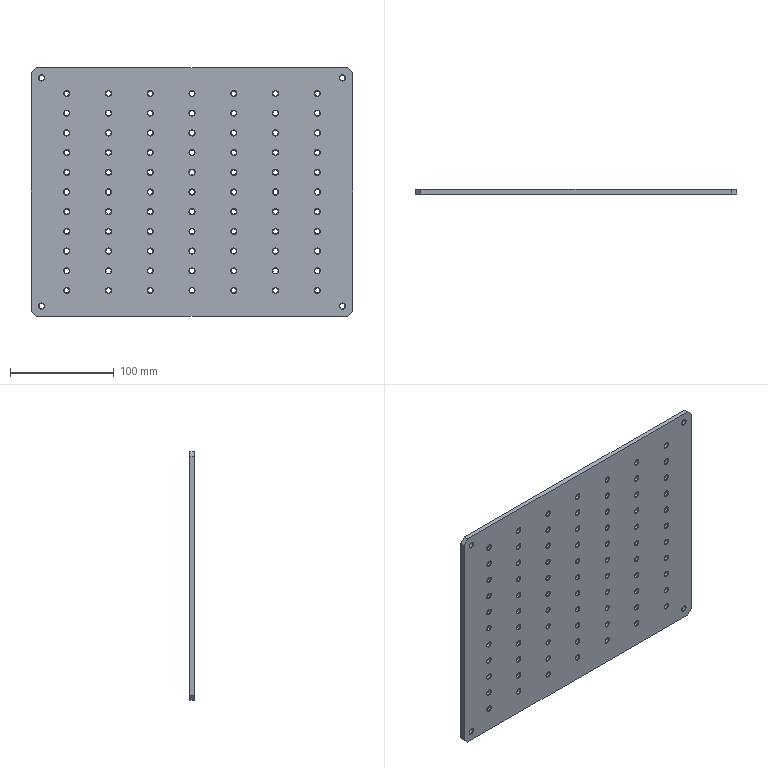Part | STEP file | Square aluminium plate (302) | 1 solid | 1728 faces | box 310 x 4.5 x 240 mm | volume 272267 mm3 | plane 780 | cylinder 624 | cone 324 | commonest cylinder face diameters 1.5 x462 5 x162